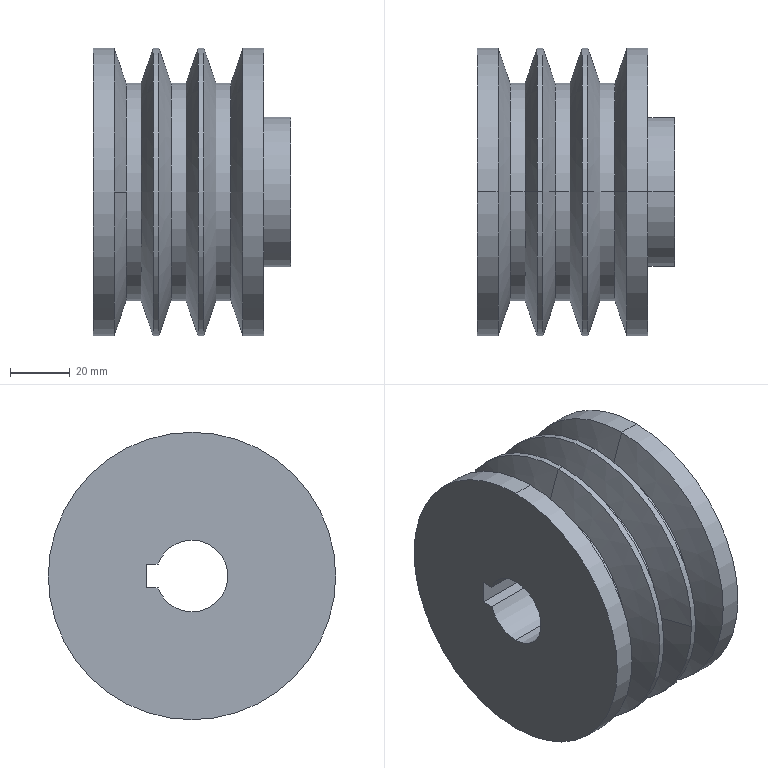Part | SolidWorks | features BaseBody 1 | 1 solid | 37 faces | box 66 x 96 x 96 mm | volume 312790 mm3 | cylinder 19 | cone 12 | plane 6 | commonest cylinder face diameters 96 x8 72.6 x6 24 x3 50 x2
STEP:
#1=CARTESIAN_POINT('',(-28.5,0.,48.));
#2=VERTEX_POINT('',#1);
#3=CARTESIAN_POINT('',(-28.5,0.,-48.));
#4=VERTEX_POINT('',#3);
#5=CARTESIAN_POINT('',(-28.5,0.,0.));
#6=DIRECTION('',(-1.,0.,0.));
#7=DIRECTION('',(0.,0.,-1.));
#8=AXIS2_PLACEMENT_3D('',#5,#6,#7);
#9=CIRCLE('',#8,48.);
#10=EDGE_CURVE('',#2,#4,#9,.T.);
#11=ORIENTED_EDGE('',*,*,#10,.F.);
#12=CARTESIAN_POINT('',(-21.533,0.,48.));
#13=VERTEX_POINT('',#12);
#14=CARTESIAN_POINT('',(0.,0.,48.));
#15=DIRECTION('',(1.,0.,0.));
#16=VECTOR('',#15,1000.);
#17=LINE('',#14,#16);
#18=EDGE_CURVE('',#2,#13,#17,.T.);
#19=ORIENTED_EDGE('',*,*,#18,.T.);
#20=CARTESIAN_POINT('',(-21.533,48.,0.));
#21=VERTEX_POINT('',#20);
#22=CARTESIAN_POINT('',(-21.533,0.,0.));
#23=DIRECTION('',(-1.,0.,0.));
#24=DIRECTION('',(0.,0.,-1.));
#25=AXIS2_PLACEMENT_3D('',#22,#23,#24);
#26=CIRCLE('',#25,48.);
#27=EDGE_CURVE('',#13,#21,#26,.T.);
#28=ORIENTED_EDGE('',*,*,#27,.T.);
#29=CARTESIAN_POINT('',(-21.533,0.,-48.));
#30=VERTEX_POINT('',#29);
#31=CARTESIAN_POINT('',(-21.533,0.,0.));
#32=DIRECTION('',(-1.,0.,0.));
#33=DIRECTION('',(0.,0.,-1.));
#34=AXIS2_PLACEMENT_3D('',#31,#32,#33);
#35=CIRCLE('',#34,48.);
#36=EDGE_CURVE('',#21,#30,#35,.T.);
#37=ORIENTED_EDGE('',*,*,#36,.T.);
#38=CARTESIAN_POINT('',(0.,0.,-48.));
#39=DIRECTION('',(1.,0.,0.));
#40=VECTOR('',#39,1000.);
#41=LINE('',#38,#40);
#42=EDGE_CURVE('',#4,#30,#41,.T.);
#43=ORIENTED_EDGE('',*,*,#42,.F.);
#44=EDGE_LOOP('',(#11,#19,#28,#37,#43));
#45=FACE_OUTER_BOUND('',#44,.T.);
#46=CARTESIAN_POINT('',(0.,0.,0.));
#47=DIRECTION('',(1.,0.,0.));
#48=DIRECTION('',(0.,0.,-1.));
#49=AXIS2_PLACEMENT_3D('',#46,#47,#48);
#50=CYLINDRICAL_SURFACE('',#49,48.);
#51=ADVANCED_FACE('',(#45),#50,.T.);
#52=CARTESIAN_POINT('',(-28.5,0.,12.));
#53=VERTEX_POINT('',#52);
#54=CARTESIAN_POINT('',(-28.5,0.,-12.));
#55=VERTEX_POINT('',#54);
#56=CARTESIAN_POINT('',(-28.5,0.,0.));
#57=DIRECTION('',(1.,0.,0.));
#58=DIRECTION('',(0.,0.,-1.));
#59=AXIS2_PLACEMENT_3D('',#56,#57,#58);
#60=CIRCLE('',#59,12.);
#61=EDGE_CURVE('',#53,#55,#60,.T.);
#62=ORIENTED_EDGE('',*,*,#61,.F.);
#63=CARTESIAN_POINT('',(37.5,0.,12.));
#64=VERTEX_POINT('',#63);
#65=CARTESIAN_POINT('',(0.,0.,12.));
#66=DIRECTION('',(1.,0.,0.));
#67=VECTOR('',#66,1000.);
#68=LINE('',#65,#67);
#69=EDGE_CURVE('',#53,#64,#68,.T.);
#70=ORIENTED_EDGE('',*,*,#69,.T.);
#71=CARTESIAN_POINT('',(37.5,0.,-12.));
#72=VERTEX_POINT('',#71);
#73=CARTESIAN_POINT('',(37.5,0.,0.));
#74=DIRECTION('',(-1.,0.,0.));
#75=DIRECTION('',(0.,0.,-1.));
#76=AXIS2_PLACEMENT_3D('',#73,#74,#75);
#77=CIRCLE('',#76,12.);
#78=EDGE_CURVE('',#72,#64,#77,.T.);
#79=ORIENTED_EDGE('',*,*,#78,.F.);
#80=CARTESIAN_POINT('',(0.,0.,-12.));
#81=DIRECTION('',(1.,0.,0.));
#82=VECTOR('',#81,1000.);
#83=LINE('',#80,#82);
#84=EDGE_CURVE('',#55,#72,#83,.T.);
#85=ORIENTED_EDGE('',*,*,#84,.F.);
#86=EDGE_LOOP('',(#62,#70,#79,#85));
#87=FACE_OUTER_BOUND('',#86,.T.);
#88=CARTESIAN_POINT('',(0.,0.,0.));
#89=DIRECTION('',(1.,0.,0.));
#90=DIRECTION('',(0.,0.,-1.));
#91=AXIS2_PLACEMENT_3D('',#88,#89,#90);
#92=CYLINDRICAL_SURFACE('',#91,12.);
#93=ADVANCED_FACE('',(#87),#92,.F.);
#94=CARTESIAN_POINT('',(-28.5,11.314,-4.));
#95=VERTEX_POINT('',#94);
#96=CARTESIAN_POINT('',(-28.5,0.,0.));
#97=DIRECTION('',(1.,0.,0.));
#98=DIRECTION('',(0.,0.,-1.));
#99=AXIS2_PLACEMENT_3D('',#96,#97,#98);
#100=CIRCLE('',#99,12.);
#101=EDGE_CURVE('',#55,#95,#100,.T.);
#102=ORIENTED_EDGE('',*,*,#101,.F.);
#103=ORIENTED_EDGE('',*,*,#84,.T.);
#104=CARTESIAN_POINT('',(37.5,11.314,-4.));
#105=VERTEX_POINT('',#104);
#106=CARTESIAN_POINT('',(37.5,0.,0.));
#107=DIRECTION('',(-1.,0.,0.));
#108=DIRECTION('',(0.,0.,-1.));
#109=AXIS2_PLACEMENT_3D('',#106,#107,#108);
#110=CIRCLE('',#109,12.);
#111=EDGE_CURVE('',#105,#72,#110,.T.);
#112=ORIENTED_EDGE('',*,*,#111,.F.);
#113=CARTESIAN_POINT('',(0.,11.314,-4.));
#114=DIRECTION('',(1.,0.,0.));
#115=VECTOR('',#114,1000.);
#116=LINE('',#113,#115);
#117=EDGE_CURVE('',#95,#105,#116,.T.);
#118=ORIENTED_EDGE('',*,*,#117,.F.);
#119=EDGE_LOOP('',(#102,#103,#112,#118));
#120=FACE_OUTER_BOUND('',#119,.T.);
#121=CARTESIAN_POINT('',(0.,0.,0.));
#122=DIRECTION('',(1.,0.,0.));
#123=DIRECTION('',(0.,0.,-1.));
#124=AXIS2_PLACEMENT_3D('',#121,#122,#123);
#125=CYLINDRICAL_SURFACE('',#124,12.);
#126=ADVANCED_FACE('',(#120),#125,.F.);
#127=CARTESIAN_POINT('',(-17.504,0.,36.3));
#128=VERTEX_POINT('',#127);
#129=CARTESIAN_POINT('',(-17.504,36.3,0.));
#130=VERTEX_POINT('',#129);
#131=CARTESIAN_POINT('',(-17.504,0.,0.));
#132=DIRECTION('',(-1.,0.,0.));
#133=DIRECTION('',(0.,0.,1.));
#134=AXIS2_PLACEMENT_3D('',#131,#132,#133);
#135=CIRCLE('',#134,36.3);
#136=EDGE_CURVE('',#128,#130,#135,.T.);
#137=ORIENTED_EDGE('',*,*,#136,.T.);
#138=CARTESIAN_POINT('',(-21.533,48.,0.));
#139=DIRECTION('',(-0.3256,0.9455,0.));
#140=VECTOR('',#139,1000.);
#141=LINE('',#138,#140);
#142=EDGE_CURVE('',#130,#21,#141,.T.);
#143=ORIENTED_EDGE('',*,*,#142,.T.);
#144=ORIENTED_EDGE('',*,*,#27,.F.);
#145=CARTESIAN_POINT('',(-21.533,-48.,0.));
#146=VERTEX_POINT('',#145);
#147=CARTESIAN_POINT('',(-21.533,0.,0.));
#148=DIRECTION('',(-1.,0.,0.));
#149=DIRECTION('',(0.,0.,-1.));
#150=AXIS2_PLACEMENT_3D('',#147,#148,#149);
#151=CIRCLE('',#150,48.);
#152=EDGE_CURVE('',#146,#13,#151,.T.);
#153=ORIENTED_EDGE('',*,*,#152,.F.);
#154=CARTESIAN_POINT('',(-17.504,-36.3,0.));
#155=VERTEX_POINT('',#154);
#156=CARTESIAN_POINT('',(-21.533,-48.,0.));
#157=DIRECTION('',(-0.3256,-0.9455,0.));
#158=VECTOR('',#157,1000.);
#159=LINE('',#156,#158);
#160=EDGE_CURVE('',#155,#146,#159,.T.);
#161=ORIENTED_EDGE('',*,*,#160,.F.);
#162=CARTESIAN_POINT('',(-17.504,0.,0.));
#163=DIRECTION('',(-1.,0.,0.));
#164=DIRECTION('',(0.,0.,1.));
#165=AXIS2_PLACEMENT_3D('',#162,#163,#164);
#166=CIRCLE('',#165,36.3);
#167=EDGE_CURVE('',#155,#128,#166,.T.);
#168=ORIENTED_EDGE('',*,*,#167,.T.);
#169=EDGE_LOOP('',(#137,#143,#144,#153,#161,#168));
#170=FACE_OUTER_BOUND('',#169,.T.);
#171=CARTESIAN_POINT('',(-21.533,0.,0.));
#172=DIRECTION('',(-1.,0.,0.));
#173=DIRECTION('',(0.,-1.,0.));
#174=AXIS2_PLACEMENT_3D('',#171,#172,#173);
#175=CONICAL_SURFACE('',#174,48.,1.239);
#176=ADVANCED_FACE('',(#170),#175,.T.);
#177=CARTESIAN_POINT('',(-12.496,0.,36.3));
#178=VERTEX_POINT('',#177);
#179=CARTESIAN_POINT('',(-12.496,0.,-36.3));
#180=VERTEX_POINT('',#179);
#181=CARTESIAN_POINT('',(-12.496,0.,0.));
#182=DIRECTION('',(-1.,0.,0.));
#183=DIRECTION('',(0.,0.,1.));
#184=AXIS2_PLACEMENT_3D('',#181,#182,#183);
#185=CIRCLE('',#184,36.3);
#186=EDGE_CURVE('',#178,#180,#185,.T.);
#187=ORIENTED_EDGE('',*,*,#186,.T.);
#188=CARTESIAN_POINT('',(-17.504,0.,-36.3));
#189=VERTEX_POINT('',#188);
#190=CARTESIAN_POINT('',(-15.,0.,-36.3));
#191=DIRECTION('',(-1.,0.,0.));
#192=VECTOR('',#191,1000.);
#193=LINE('',#190,#192);
#194=EDGE_CURVE('',#180,#189,#193,.T.);
#195=ORIENTED_EDGE('',*,*,#194,.T.);
#196=CARTESIAN_POINT('',(-17.504,0.,0.));
#197=DIRECTION('',(-1.,0.,0.));
#198=DIRECTION('',(0.,0.,1.));
#199=AXIS2_PLACEMENT_3D('',#196,#197,#198);
#200=CIRCLE('',#199,36.3);
#201=EDGE_CURVE('',#130,#189,#200,.T.);
#202=ORIENTED_EDGE('',*,*,#201,.F.);
#203=ORIENTED_EDGE('',*,*,#136,.F.);
#204=CARTESIAN_POINT('',(-15.,0.,36.3));
#205=DIRECTION('',(-1.,0.,0.));
#206=VECTOR('',#205,1000.);
#207=LINE('',#204,#206);
#208=EDGE_CURVE('',#178,#128,#207,.T.);
#209=ORIENTED_EDGE('',*,*,#208,.F.);
#210=EDGE_LOOP('',(#187,#195,#202,#203,#209));
#211=FACE_OUTER_BOUND('',#210,.T.);
#212=CARTESIAN_POINT('',(-15.,0.,0.));
#213=DIRECTION('',(-1.,0.,0.));
#214=DIRECTION('',(0.,0.,1.));
#215=AXIS2_PLACEMENT_3D('',#212,#213,#214);
#216=CYLINDRICAL_SURFACE('',#215,36.3);
#217=ADVANCED_FACE('',(#211),#216,.T.);
#218=CARTESIAN_POINT('',(28.5,0.,-25.));
#219=VERTEX_POINT('',#218);
#220=CARTESIAN_POINT('',(28.5,0.,25.));
#221=VERTEX_POINT('',#220);
#222=CARTESIAN_POINT('',(28.5,0.,0.));
#223=DIRECTION('',(1.,0.,0.));
#224=DIRECTION('',(0.,0.,-1.));
#225=AXIS2_PLACEMENT_3D('',#222,#223,#224);
#226=CIRCLE('',#225,25.);
#227=EDGE_CURVE('',#219,#221,#226,.T.);
#228=ORIENTED_EDGE('',*,*,#227,.T.);
#229=CARTESIAN_POINT('',(37.5,0.,25.));
#230=VERTEX_POINT('',#229);
#231=CARTESIAN_POINT('',(0.,0.,25.));
#232=DIRECTION('',(1.,0.,0.));
#233=VECTOR('',#232,1000.);
#234=LINE('',#231,#233);
#235=EDGE_CURVE('',#221,#230,#234,.T.);
#236=ORIENTED_EDGE('',*,*,#235,.T.);
#237=CARTESIAN_POINT('',(37.5,0.,-25.));
#238=VERTEX_POINT('',#237);
#239=CARTESIAN_POINT('',(37.5,0.,0.));
#240=DIRECTION('',(1.,0.,0.));
#241=DIRECTION('',(0.,0.,-1.));
#242=AXIS2_PLACEMENT_3D('',#239,#240,#241);
#243=CIRCLE('',#242,25.);
#244=EDGE_CURVE('',#238,#230,#243,.T.);
#245=ORIENTED_EDGE('',*,*,#244,.F.);
#246=CARTESIAN_POINT('',(0.,0.,-25.));
#247=DIRECTION('',(1.,0.,0.));
#248=VECTOR('',#247,1000.);
#249=LINE('',#246,#248);
#250=EDGE_CURVE('',#219,#238,#249,.T.);
#251=ORIENTED_EDGE('',*,*,#250,.F.);
#252=EDGE_LOOP('',(#228,#236,#245,#251));
#253=FACE_OUTER_BOUND('',#252,.T.);
#254=CARTESIAN_POINT('',(0.,0.,0.));
#255=DIRECTION('',(1.,0.,0.));
#256=DIRECTION('',(0.,0.,-1.));
#257=AXIS2_PLACEMENT_3D('',#254,#255,#256);
#258=CYLINDRICAL_SURFACE('',#257,25.);
#259=ADVANCED_FACE('',(#253),#258,.T.);
#260=ORIENTED_EDGE('',*,*,#186,.F.);
#261=CARTESIAN_POINT('',(-8.467,0.,48.));
#262=VERTEX_POINT('',#261);
#263=CARTESIAN_POINT('',(-8.467,0.,48.));
#264=DIRECTION('',(0.3256,0.,0.9455));
#265=VECTOR('',#264,1000.);
#266=LINE('',#263,#265);
#267=EDGE_CURVE('',#178,#262,#266,.T.);
#268=ORIENTED_EDGE('',*,*,#267,.T.);
#269=CARTESIAN_POINT('',(-8.467,0.,-48.));
#270=VERTEX_POINT('',#269);
#271=CARTESIAN_POINT('',(-8.467,0.,0.));
#272=DIRECTION('',(-1.,0.,0.));
#273=DIRECTION('',(0.,0.,-1.));
#274=AXIS2_PLACEMENT_3D('',#271,#272,#273);
#275=CIRCLE('',#274,48.);
#276=EDGE_CURVE('',#262,#270,#275,.T.);
#277=ORIENTED_EDGE('',*,*,#276,.T.);
#278=CARTESIAN_POINT('',(-8.467,0.,-48.));
#279=DIRECTION('',(0.3256,0.,-0.9455));
#280=VECTOR('',#279,1000.);
#281=LINE('',#278,#280);
#282=EDGE_CURVE('',#180,#270,#281,.T.);
#283=ORIENTED_EDGE('',*,*,#282,.F.);
#284=EDGE_LOOP('',(#260,#268,#277,#283));
#285=FACE_OUTER_BOUND('',#284,.T.);
#286=CARTESIAN_POINT('',(-8.467,0.,0.));
#287=DIRECTION('',(1.,0.,0.));
#288=DIRECTION('',(0.,0.,-1.));
#289=AXIS2_PLACEMENT_3D('',#286,#287,#288);
#290=CONICAL_SURFACE('',#289,48.,1.239);
#291=ADVANCED_FACE('',(#285),#290,.T.);
#292=ORIENTED_EDGE('',*,*,#276,.F.);
#293=CARTESIAN_POINT('',(-6.533,0.,48.));
#294=VERTEX_POINT('',#293);
#295=CARTESIAN_POINT('',(0.,0.,48.));
#296=DIRECTION('',(1.,0.,0.));
#297=VECTOR('',#296,1000.);
#298=LINE('',#295,#297);
#299=EDGE_CURVE('',#262,#294,#298,.T.);
#300=ORIENTED_EDGE('',*,*,#299,.T.);
#301=CARTESIAN_POINT('',(-6.533,0.,-48.));
#302=VERTEX_POINT('',#301);
#303=CARTESIAN_POINT('',(-6.533,0.,0.));
#304=DIRECTION('',(-1.,0.,0.));
#305=DIRECTION('',(0.,0.,-1.));
#306=AXIS2_PLACEMENT_3D('',#303,#304,#305);
#307=CIRCLE('',#306,48.);
#308=EDGE_CURVE('',#294,#302,#307,.T.);
#309=ORIENTED_EDGE('',*,*,#308,.T.);
#310=CARTESIAN_POINT('',(0.,0.,-48.));
#311=DIRECTION('',(1.,0.,0.));
#312=VECTOR('',#311,1000.);
#313=LINE('',#310,#312);
#314=EDGE_CURVE('',#270,#302,#313,.T.);
#315=ORIENTED_EDGE('',*,*,#314,.F.);
#316=EDGE_LOOP('',(#292,#300,#309,#315));
#317=FACE_OUTER_BOUND('',#316,.T.);
#318=CARTESIAN_POINT('',(0.,0.,0.));
#319=DIRECTION('',(1.,0.,0.));
#320=DIRECTION('',(0.,0.,-1.));
#321=AXIS2_PLACEMENT_3D('',#318,#319,#320);
#322=CYLINDRICAL_SURFACE('',#321,48.);
#323=ADVANCED_FACE('',(#317),#322,.T.);
#324=CARTESIAN_POINT('',(21.533,0.,-48.));
#325=VERTEX_POINT('',#324);
#326=CARTESIAN_POINT('',(21.533,0.,48.));
#327=VERTEX_POINT('',#326);
#328=CARTESIAN_POINT('',(21.533,0.,0.));
#329=DIRECTION('',(1.,0.,0.));
#330=DIRECTION('',(0.,0.,-1.));
#331=AXIS2_PLACEMENT_3D('',#328,#329,#330);
#332=CIRCLE('',#331,48.);
#333=EDGE_CURVE('',#325,#327,#332,.T.);
#334=ORIENTED_EDGE('',*,*,#333,.T.);
#335=CARTESIAN_POINT('',(28.5,0.,48.));
#336=VERTEX_POINT('',#335);
#337=CARTESIAN_POINT('',(0.,0.,48.));
#338=DIRECTION('',(1.,0.,0.));
#339=VECTOR('',#338,1000.);
#340=LINE('',#337,#339);
#341=EDGE_CURVE('',#327,#336,#340,.T.);
#342=ORIENTED_EDGE('',*,*,#341,.T.);
#343=CARTESIAN_POINT('',(28.5,0.,-48.));
#344=VERTEX_POINT('',#343);
#345=CARTESIAN_POINT('',(28.5,0.,0.));
#346=DIRECTION('',(1.,0.,0.));
#347=DIRECTION('',(0.,0.,-1.));
#348=AXIS2_PLACEMENT_3D('',#345,#346,#347);
#349=CIRCLE('',#348,48.);
#350=EDGE_CURVE('',#344,#336,#349,.T.);
#351=ORIENTED_EDGE('',*,*,#350,.F.);
#352=CARTESIAN_POINT('',(0.,0.,-48.));
#353=DIRECTION('',(1.,0.,0.));
#354=VECTOR('',#353,1000.);
#355=LINE('',#352,#354);
#356=EDGE_CURVE('',#325,#344,#355,.T.);
#357=ORIENTED_EDGE('',*,*,#356,.F.);
#358=EDGE_LOOP('',(#334,#342,#351,#357));
#359=FACE_OUTER_BOUND('',#358,.T.);
#360=CARTESIAN_POINT('',(0.,0.,0.));
#361=DIRECTION('',(1.,0.,0.));
#362=DIRECTION('',(0.,0.,-1.));
#363=AXIS2_PLACEMENT_3D('',#360,#361,#362);
#364=CYLINDRICAL_SURFACE('',#363,48.);
#365=ADVANCED_FACE('',(#359),#364,.T.);
#366=CARTESIAN_POINT('',(-2.504,0.,36.3));
#367=VERTEX_POINT('',#366);
#368=CARTESIAN_POINT('',(-2.504,0.,-36.3));
#369=VERTEX_POINT('',#368);
#370=CARTESIAN_POINT('',(-2.504,0.,0.));
#371=DIRECTION('',(-1.,0.,0.));
#372=DIRECTION('',(0.,0.,1.));
#373=AXIS2_PLACEMENT_3D('',#370,#371,#372);
#374=CIRCLE('',#373,36.3);
#375=EDGE_CURVE('',#367,#369,#374,.T.);
#376=ORIENTED_EDGE('',*,*,#375,.T.);
#377=CARTESIAN_POINT('',(-6.533,0.,-48.));
#378=DIRECTION('',(-0.3256,0.,-0.9455));
#379=VECTOR('',#378,1000.);
#380=LINE('',#377,#379);
#381=EDGE_CURVE('',#369,#302,#380,.T.);
#382=ORIENTED_EDGE('',*,*,#381,.T.);
#383=ORIENTED_EDGE('',*,*,#308,.F.);
#384=CARTESIAN_POINT('',(-6.533,0.,48.));
#385=DIRECTION('',(-0.3256,0.,0.9455));
#386=VECTOR('',#385,1000.);
#387=LINE('',#384,#386);
#388=EDGE_CURVE('',#367,#294,#387,.T.);
#389=ORIENTED_EDGE('',*,*,#388,.F.);
#390=EDGE_LOOP('',(#376,#382,#383,#389));
#391=FACE_OUTER_BOUND('',#390,.T.);
#392=CARTESIAN_POINT('',(-6.533,0.,0.));
#393=DIRECTION('',(-1.,0.,0.));
#394=DIRECTION('',(0.,0.,1.));
#395=AXIS2_PLACEMENT_3D('',#392,#393,#394);
#396=CONICAL_SURFACE('',#395,48.,1.239);
#397=ADVANCED_FACE('',(#391),#396,.T.);
#398=CARTESIAN_POINT('',(17.504,0.,-36.3));
#399=VERTEX_POINT('',#398);
#400=CARTESIAN_POINT('',(17.504,0.,36.3));
#401=VERTEX_POINT('',#400);
#402=CARTESIAN_POINT('',(17.504,0.,0.));
#403=DIRECTION('',(1.,0.,0.));
#404=DIRECTION('',(0.,0.,-1.));
#405=AXIS2_PLACEMENT_3D('',#402,#403,#404);
#406=CIRCLE('',#405,36.3);
#407=EDGE_CURVE('',#399,#401,#406,.T.);
#408=ORIENTED_EDGE('',*,*,#407,.T.);
#409=CARTESIAN_POINT('',(21.533,0.,48.));
#410=DIRECTION('',(0.3256,0.,0.9455));
#411=VECTOR('',#410,1000.);
#412=LINE('',#409,#411);
#413=EDGE_CURVE('',#401,#327,#412,.T.);
#414=ORIENTED_EDGE('',*,*,#413,.T.);
#415=ORIENTED_EDGE('',*,*,#333,.F.);
#416=CARTESIAN_POINT('',(21.533,0.,-48.));
#417=DIRECTION('',(0.3256,0.,-0.9455));
#418=VECTOR('',#417,1000.);
#419=LINE('',#416,#418);
#420=EDGE_CURVE('',#399,#325,#419,.T.);
#421=ORIENTED_EDGE('',*,*,#420,.F.);
#422=EDGE_LOOP('',(#408,#414,#415,#421));
#423=FACE_OUTER_BOUND('',#422,.T.);
#424=CARTESIAN_POINT('',(21.533,0.,0.));
#425=DIRECTION('',(1.,0.,0.));
#426=DIRECTION('',(0.,0.,-1.));
#427=AXIS2_PLACEMENT_3D('',#424,#425,#426);
#428=CONICAL_SURFACE('',#427,48.,1.239);
#429=ADVANCED_FACE('',(#423),#428,.T.);
#430=CARTESIAN_POINT('',(2.504,36.3,0.));
#431=VERTEX_POINT('',#430);
#432=CARTESIAN_POINT('',(2.504,0.,-36.3));
#433=VERTEX_POINT('',#432);
#434=CARTESIAN_POINT('',(2.504,0.,0.));
#435=DIRECTION('',(-1.,0.,0.));
#436=DIRECTION('',(0.,0.,1.));
#437=AXIS2_PLACEMENT_3D('',#434,#435,#436);
#438=CIRCLE('',#437,36.3);
#439=EDGE_CURVE('',#431,#433,#438,.T.);
#440=ORIENTED_EDGE('',*,*,#439,.T.);
#441=CARTESIAN_POINT('',(0.,0.,-36.3));
#442=DIRECTION('',(-1.,0.,0.));
#443=VECTOR('',#442,1000.);
#444=LINE('',#441,#443);
#445=EDGE_CURVE('',#433,#369,#444,.T.);
#446=ORIENTED_EDGE('',*,*,#445,.T.);
#447=ORIENTED_EDGE('',*,*,#375,.F.);
#448=CARTESIAN_POINT('',(2.504,0.,36.3));
#449=VERTEX_POINT('',#448);
#450=CARTESIAN_POINT('',(0.,0.,36.3));
#451=DIRECTION('',(-1.,0.,0.));
#452=VECTOR('',#451,1000.);
#453=LINE('',#450,#452);
#454=EDGE_CURVE('',#449,#367,#453,.T.);
#455=ORIENTED_EDGE('',*,*,#454,.F.);
#456=CARTESIAN_POINT('',(2.504,0.,0.));
#457=DIRECTION('',(-1.,0.,0.));
#458=DIRECTION('',(0.,0.,1.));
#459=AXIS2_PLACEMENT_3D('',#456,#457,#458);
#460=CIRCLE('',#459,36.3);
#461=EDGE_CURVE('',#449,#431,#460,.T.);
#462=ORIENTED_EDGE('',*,*,#461,.T.);
#463=EDGE_LOOP('',(#440,#446,#447,#455,#462));
#464=FACE_OUTER_BOUND('',#463,.T.);
#465=CARTESIAN_POINT('',(0.,0.,0.));
#466=DIRECTION('',(-1.,0.,0.));
#467=DIRECTION('',(0.,0.,1.));
#468=AXIS2_PLACEMENT_3D('',#465,#466,#467);
#469=CYLINDRICAL_SURFACE('',#468,36.3);
#470=ADVANCED_FACE('',(#464),#469,.T.);
#471=ORIENTED_EDGE('',*,*,#407,.F.);
#472=CARTESIAN_POINT('',(12.496,0.,-36.3));
#473=VERTEX_POINT('',#472);
#474=CARTESIAN_POINT('',(15.,0.,-36.3));
#475=DIRECTION('',(-1.,0.,0.));
#476=VECTOR('',#475,1000.);
#477=LINE('',#474,#476);
#478=EDGE_CURVE('',#399,#473,#477,.T.);
#479=ORIENTED_EDGE('',*,*,#478,.T.);
#480=CARTESIAN_POINT('',(12.496,0.,36.3));
#481=VERTEX_POINT('',#480);
#482=CARTESIAN_POINT('',(12.496,0.,0.));
#483=DIRECTION('',(1.,0.,0.));
#484=DIRECTION('',(0.,0.,1.));
#485=AXIS2_PLACEMENT_3D('',#482,#483,#484);
#486=CIRCLE('',#485,36.3);
#487=EDGE_CURVE('',#473,#481,#486,.T.);
#488=ORIENTED_EDGE('',*,*,#487,.T.);
#489=CARTESIAN_POINT('',(15.,0.,36.3));
#490=DIRECTION('',(-1.,0.,0.));
#491=VECTOR('',#490,1000.);
#492=LINE('',#489,#491);
#493=EDGE_CURVE('',#401,#481,#492,.T.);
#494=ORIENTED_EDGE('',*,*,#493,.F.);
#495=EDGE_LOOP('',(#471,#479,#488,#494));
#496=FACE_OUTER_BOUND('',#495,.T.);
#497=CARTESIAN_POINT('',(15.,0.,0.));
#498=DIRECTION('',(-1.,0.,0.));
#499=DIRECTION('',(0.,0.,1.));
#500=AXIS2_PLACEMENT_3D('',#497,#498,#499);
#501=CYLINDRICAL_SURFACE('',#500,36.3);
#502=ADVANCED_FACE('',(#496),#501,.T.);
#503=CARTESIAN_POINT('',(2.504,-36.3,0.));
#504=VERTEX_POINT('',#503);
#505=CARTESIAN_POINT('',(2.504,0.,0.));
#506=DIRECTION('',(-1.,0.,0.));
#507=DIRECTION('',(0.,0.,1.));
#508=AXIS2_PLACEMENT_3D('',#505,#506,#507);
#509=CIRCLE('',#508,36.3);
#510=EDGE_CURVE('',#504,#449,#509,.T.);
#511=ORIENTED_EDGE('',*,*,#510,.F.);
#512=CARTESIAN_POINT('',(6.533,-48.,0.));
#513=VERTEX_POINT('',#512);
#514=CARTESIAN_POINT('',(6.533,-48.,0.));
#515=DIRECTION('',(0.3256,-0.9455,0.));
#516=VECTOR('',#515,1000.);
#517=LINE('',#514,#516);
#518=EDGE_CURVE('',#504,#513,#517,.T.);
#519=ORIENTED_EDGE('',*,*,#518,.T.);
#520=CARTESIAN_POINT('',(6.533,0.,48.));
#521=VERTEX_POINT('',#520);
#522=CARTESIAN_POINT('',(6.533,0.,0.));
#523=DIRECTION('',(-1.,0.,0.));
#524=DIRECTION('',(0.,0.,-1.));
#525=AXIS2_PLACEMENT_3D('',#522,#523,#524);
#526=CIRCLE('',#525,48.);
#527=EDGE_CURVE('',#513,#521,#526,.T.);
#528=ORIENTED_EDGE('',*,*,#527,.T.);
#529=CARTESIAN_POINT('',(6.533,48.,0.));
#530=VERTEX_POINT('',#529);
#531=CARTESIAN_POINT('',(6.533,0.,0.));
#532=DIRECTION('',(-1.,0.,0.));
#533=DIRECTION('',(0.,0.,-1.));
#534=AXIS2_PLACEMENT_3D('',#531,#532,#533);
#535=CIRCLE('',#534,48.);
#536=EDGE_CURVE('',#521,#530,#535,.T.);
#537=ORIENTED_EDGE('',*,*,#536,.T.);
#538=CARTESIAN_POINT('',(6.533,48.,0.));
#539=DIRECTION('',(0.3256,0.9455,0.));
#540=VECTOR('',#539,1000.);
#541=LINE('',#538,#540);
#542=EDGE_CURVE('',#431,#530,#541,.T.);
#543=ORIENTED_EDGE('',*,*,#542,.F.);
#544=ORIENTED_EDGE('',*,*,#461,.F.);
#545=EDGE_LOOP('',(#511,#519,#528,#537,#543,#544));
#546=FACE_OUTER_BOUND('',#545,.T.);
#547=CARTESIAN_POINT('',(6.533,0.,0.));
#548=DIRECTION('',(1.,0.,0.));
#549=DIRECTION('',(0.,1.,0.));
#550=AXIS2_PLACEMENT_3D('',#547,#548,#549);
#551=CONICAL_SURFACE('',#550,48.,1.239);
#552=ADVANCED_FACE('',(#546),#551,.T.);
#553=ORIENTED_EDGE('',*,*,#487,.F.);
#554=CARTESIAN_POINT('',(8.467,0.,-48.));
#555=VERTEX_POINT('',#554);
#556=CARTESIAN_POINT('',(8.467,0.,-48.));
#557=DIRECTION('',(-0.3256,0.,-0.9455));
#558=VECTOR('',#557,1000.);
#559=LINE('',#556,#558);
#560=EDGE_CURVE('',#473,#555,#559,.T.);
#561=ORIENTED_EDGE('',*,*,#560,.T.);
#562=CARTESIAN_POINT('',(8.467,0.,48.));
#563=VERTEX_POINT('',#562);
#564=CARTESIAN_POINT('',(8.467,0.,0.));
#565=DIRECTION('',(1.,0.,0.));
#566=DIRECTION('',(0.,0.,1.));
#567=AXIS2_PLACEMENT_3D('',#564,#565,#566);
#568=CIRCLE('',#567,48.);
#569=EDGE_CURVE('',#555,#563,#568,.T.);
#570=ORIENTED_EDGE('',*,*,#569,.T.);
#571=CARTESIAN_POINT('',(8.467,0.,48.));
#572=DIRECTION('',(-0.3256,0.,0.9455));
#573=VECTOR('',#572,1000.);
#574=LINE('',#571,#573);
#575=EDGE_CURVE('',#481,#563,#574,.T.);
#576=ORIENTED_EDGE('',*,*,#575,.F.);
#577=EDGE_LOOP('',(#553,#561,#570,#576));
#578=FACE_OUTER_BOUND('',#577,.T.);
#579=CARTESIAN_POINT('',(8.467,0.,0.));
#580=DIRECTION('',(-1.,0.,0.));
#581=DIRECTION('',(0.,0.,1.));
#582=AXIS2_PLACEMENT_3D('',#579,#580,#581);
#583=CONICAL_SURFACE('',#582,48.,1.239);
#584=ADVANCED_FACE('',(#578),#583,.T.);
#585=ORIENTED_EDGE('',*,*,#536,.F.);
#586=CARTESIAN_POINT('',(0.,0.,48.));
#587=DIRECTION('',(1.,0.,0.));
#588=VECTOR('',#587,1000.);
#589=LINE('',#586,#588);
#590=EDGE_CURVE('',#521,#563,#589,.T.);
#591=ORIENTED_EDGE('',*,*,#590,.T.);
#592=ORIENTED_EDGE('',*,*,#569,.F.);
#593=CARTESIAN_POINT('',(6.533,0.,-48.));
#594=VERTEX_POINT('',#593);
#595=CARTESIAN_POINT('',(0.,0.,-48.));
#596=DIRECTION('',(1.,0.,0.));
#597=VECTOR('',#596,1000.);
#598=LINE('',#595,#597);
#599=EDGE_CURVE('',#594,#555,#598,.T.);
#600=ORIENTED_EDGE('',*,*,#599,.F.);
#601=CARTESIAN_POINT('',(6.533,0.,0.));
#602=DIRECTION('',(-1.,0.,0.));
#603=DIRECTION('',(0.,0.,-1.));
#604=AXIS2_PLACEMENT_3D('',#601,#602,#603);
#605=CIRCLE('',#604,48.);
#606=EDGE_CURVE('',#530,#594,#605,.T.);
#607=ORIENTED_EDGE('',*,*,#606,.F.);
#608=EDGE_LOOP('',(#585,#591,#592,#600,#607));
#609=FACE_OUTER_BOUND('',#608,.T.);
#610=CARTESIAN_POINT('',(0.,0.,0.));
#611=DIRECTION('',(1.,0.,0.));
#612=DIRECTION('',(0.,0.,-1.));
#613=AXIS2_PLACEMENT_3D('',#610,#611,#612);
#614=CYLINDRICAL_SURFACE('',#613,48.);
#615=ADVANCED_FACE('',(#609),#614,.T.);
#616=CARTESIAN_POINT('',(-28.5,0.,0.));
#617=DIRECTION('',(-1.,0.,0.));
#618=DIRECTION('',(0.,0.,-1.));
#619=AXIS2_PLACEMENT_3D('',#616,#617,#618);
#620=CIRCLE('',#619,48.);
#621=EDGE_CURVE('',#4,#2,#620,.T.);
#622=ORIENTED_EDGE('',*,*,#621,.T.);
#623=ORIENTED_EDGE('',*,*,#10,.T.);
#624=EDGE_LOOP('',(#622,#623));
#625=FACE_OUTER_BOUND('',#624,.T.);
#626=CARTESIAN_POINT('',(-28.5,11.314,4.));
#627=VERTEX_POINT('',#626);
#628=CARTESIAN_POINT('',(-28.5,0.,0.));
#629=DIRECTION('',(1.,0.,0.));
#630=DIRECTION('',(0.,0.,-1.));
#631=AXIS2_PLACEMENT_3D('',#628,#629,#630);
#632=CIRCLE('',#631,12.);
#633=EDGE_CURVE('',#627,#53,#632,.T.);
#634=ORIENTED_EDGE('',*,*,#633,.T.);
#635=ORIENTED_EDGE('',*,*,#61,.T.);
#636=ORIENTED_EDGE('',*,*,#101,.T.);
#637=CARTESIAN_POINT('',(-28.5,15.3,-4.));
#638=VERTEX_POINT('',#637);
#639=CARTESIAN_POINT('',(-28.5,48.,-4.));
#640=DIRECTION('',(0.,1.,0.));
#641=VECTOR('',#640,1000.);
#642=LINE('',#639,#641);
#643=EDGE_CURVE('',#95,#638,#642,.T.);
#644=ORIENTED_EDGE('',*,*,#643,.T.);
#645=CARTESIAN_POINT('',(-28.5,15.3,4.));
#646=VERTEX_POINT('',#645);
#647=CARTESIAN_POINT('',(-28.5,15.3,0.));
#648=DIRECTION('',(0.,0.,1.));
#649=VECTOR('',#648,1000.);
#650=LINE('',#647,#649);
#651=EDGE_CURVE('',#638,#646,#650,.T.);
#652=ORIENTED_EDGE('',*,*,#651,.T.);
#653=CARTESIAN_POINT('',(-28.5,48.,4.));
#654=DIRECTION('',(0.,-1.,0.));
#655=VECTOR('',#654,1000.);
#656=LINE('',#653,#655);
#657=EDGE_CURVE('',#646,#627,#656,.T.);
#658=ORIENTED_EDGE('',*,*,#657,.T.);
#659=EDGE_LOOP('',(#634,#635,#636,#644,#652,#658));
#660=FACE_BOUND('',#659,.T.);
#661=CARTESIAN_POINT('',(-28.5,48.,0.));
#662=DIRECTION('',(-1.,0.,0.));
#663=DIRECTION('',(0.,0.,1.));
#664=AXIS2_PLACEMENT_3D('',#661,#662,#663);
#665=PLANE('',#664);
#666=ADVANCED_FACE('',(#625,#660),#665,.T.);
#667=ORIENTED_EDGE('',*,*,#18,.F.);
#668=ORIENTED_EDGE('',*,*,#621,.F.);
#669=ORIENTED_EDGE('',*,*,#42,.T.);
#670=CARTESIAN_POINT('',(-21.533,0.,0.));
#671=DIRECTION('',(-1.,0.,0.));
#672=DIRECTION('',(0.,0.,-1.));
#673=AXIS2_PLACEMENT_3D('',#670,#671,#672);
#674=CIRCLE('',#673,48.);
#675=EDGE_CURVE('',#30,#146,#674,.T.);
#676=ORIENTED_EDGE('',*,*,#675,.T.);
#677=ORIENTED_EDGE('',*,*,#152,.T.);
#678=EDGE_LOOP('',(#667,#668,#669,#676,#677));
#679=FACE_OUTER_BOUND('',#678,.T.);
#680=CARTESIAN_POINT('',(0.,0.,0.));
#681=DIRECTION('',(1.,0.,0.));
#682=DIRECTION('',(0.,0.,-1.));
#683=AXIS2_PLACEMENT_3D('',#680,#681,#682);
#684=CYLINDRICAL_SURFACE('',#683,48.);
#685=ADVANCED_FACE('',(#679),#684,.T.);
#686=ORIENTED_EDGE('',*,*,#69,.F.);
#687=ORIENTED_EDGE('',*,*,#633,.F.);
#688=CARTESIAN_POINT('',(37.5,11.314,4.));
#689=VERTEX_POINT('',#688);
#690=CARTESIAN_POINT('',(0.,11.314,4.));
#691=DIRECTION('',(-1.,0.,0.));
#692=VECTOR('',#691,1000.);
#693=LINE('',#690,#692);
#694=EDGE_CURVE('',#689,#627,#693,.T.);
#695=ORIENTED_EDGE('',*,*,#694,.F.);
#696=CARTESIAN_POINT('',(37.5,0.,0.));
#697=DIRECTION('',(-1.,0.,0.));
#698=DIRECTION('',(0.,0.,-1.));
#699=AXIS2_PLACEMENT_3D('',#696,#697,#698);
#700=CIRCLE('',#699,12.);
#701=EDGE_CURVE('',#64,#689,#700,.T.);
#702=ORIENTED_EDGE('',*,*,#701,.F.);
#703=EDGE_LOOP('',(#686,#687,#695,#702));
#704=FACE_OUTER_BOUND('',#703,.T.);
#705=CARTESIAN_POINT('',(0.,0.,0.));
#706=DIRECTION('',(1.,0.,0.));
#707=DIRECTION('',(0.,0.,-1.));
#708=AXIS2_PLACEMENT_3D('',#705,#706,#707);
#709=CYLINDRICAL_SURFACE('',#708,12.);
#710=ADVANCED_FACE('',(#704),#709,.F.);
#711=ORIENTED_EDGE('',*,*,#657,.F.);
#712=CARTESIAN_POINT('',(37.5,15.3,4.));
#713=VERTEX_POINT('',#712);
#714=CARTESIAN_POINT('',(-28.5,15.3,4.));
#715=DIRECTION('',(-1.,0.,0.));
#716=VECTOR('',#715,1000.);
#717=LINE('',#714,#716);
#718=EDGE_CURVE('',#713,#646,#717,.T.);
#719=ORIENTED_EDGE('',*,*,#718,.F.);
#720=CARTESIAN_POINT('',(37.5,8.7,4.));
#721=DIRECTION('',(0.,1.,0.));
#722=VECTOR('',#721,1000.);
#723=LINE('',#720,#722);
#724=EDGE_CURVE('',#689,#713,#723,.T.);
#725=ORIENTED_EDGE('',*,*,#724,.F.);
#726=ORIENTED_EDGE('',*,*,#694,.T.);
#727=EDGE_LOOP('',(#711,#719,#725,#726));
#728=FACE_OUTER_BOUND('',#727,.T.);
#729=CARTESIAN_POINT('',(-28.5,8.7,4.));
#730=DIRECTION('',(0.,0.,1.));
#731=DIRECTION('',(1.,0.,0.));
#732=AXIS2_PLACEMENT_3D('',#729,#730,#731);
#733=PLANE('',#732);
#734=ADVANCED_FACE('',(#728),#733,.F.);
#735=ORIENTED_EDGE('',*,*,#718,.T.);
#736=ORIENTED_EDGE('',*,*,#651,.F.);
#737=CARTESIAN_POINT('',(37.5,15.3,-4.));
#738=VERTEX_POINT('',#737);
#739=CARTESIAN_POINT('',(-28.5,15.3,-4.));
#740=DIRECTION('',(-1.,0.,0.));
#741=VECTOR('',#740,1000.);
#742=LINE('',#739,#741);
#743=EDGE_CURVE('',#738,#638,#742,.T.);
#744=ORIENTED_EDGE('',*,*,#743,.F.);
#745=CARTESIAN_POINT('',(37.5,15.3,4.));
#746=DIRECTION('',(0.,0.,-1.));
#747=VECTOR('',#746,1000.);
#748=LINE('',#745,#747);
#749=EDGE_CURVE('',#713,#738,#748,.T.);
#750=ORIENTED_EDGE('',*,*,#749,.F.);
#751=EDGE_LOOP('',(#735,#736,#744,#750));
#752=FACE_OUTER_BOUND('',#751,.T.);
#753=CARTESIAN_POINT('',(-28.5,15.3,4.));
#754=DIRECTION('',(0.,1.,0.));
#755=DIRECTION('',(0.,0.,1.));
#756=AXIS2_PLACEMENT_3D('',#753,#754,#755);
#757=PLANE('',#756);
#758=ADVANCED_FACE('',(#752),#757,.F.);
#759=CARTESIAN_POINT('',(37.5,8.7,-4.));
#760=DIRECTION('',(0.,-1.,0.));
#761=VECTOR('',#760,1000.);
#762=LINE('',#759,#761);
#763=EDGE_CURVE('',#738,#105,#762,.T.);
#764=ORIENTED_EDGE('',*,*,#763,.F.);
#765=ORIENTED_EDGE('',*,*,#743,.T.);
#766=ORIENTED_EDGE('',*,*,#643,.F.);
#767=ORIENTED_EDGE('',*,*,#117,.T.);
#768=EDGE_LOOP('',(#764,#765,#766,#767));
#769=FACE_OUTER_BOUND('',#768,.T.);
#770=CARTESIAN_POINT('',(-28.5,8.7,-4.));
#771=DIRECTION('',(0.,0.,-1.));
#772=DIRECTION('',(-1.,0.,0.));
#773=AXIS2_PLACEMENT_3D('',#770,#771,#772);
#774=PLANE('',#773);
#775=ADVANCED_FACE('',(#769),#774,.F.);
#776=ORIENTED_EDGE('',*,*,#142,.F.);
#777=ORIENTED_EDGE('',*,*,#201,.T.);
#778=CARTESIAN_POINT('',(-17.504,0.,0.));
#779=DIRECTION('',(-1.,0.,0.));
#780=DIRECTION('',(0.,0.,1.));
#781=AXIS2_PLACEMENT_3D('',#778,#779,#780);
#782=CIRCLE('',#781,36.3);
#783=EDGE_CURVE('',#189,#155,#782,.T.);
#784=ORIENTED_EDGE('',*,*,#783,.T.);
#785=ORIENTED_EDGE('',*,*,#160,.T.);
#786=ORIENTED_EDGE('',*,*,#675,.F.);
#787=ORIENTED_EDGE('',*,*,#36,.F.);
#788=EDGE_LOOP('',(#776,#777,#784,#785,#786,#787));
#789=FACE_OUTER_BOUND('',#788,.T.);
#790=CARTESIAN_POINT('',(-21.533,0.,0.));
#791=DIRECTION('',(-1.,0.,0.));
#792=DIRECTION('',(0.,-1.,0.));
#793=AXIS2_PLACEMENT_3D('',#790,#791,#792);
#794=CONICAL_SURFACE('',#793,48.,1.239);
#795=ADVANCED_FACE('',(#789),#794,.T.);
#796=ORIENTED_EDGE('',*,*,#244,.T.);
#797=CARTESIAN_POINT('',(37.5,0.,0.));
#798=DIRECTION('',(1.,0.,0.));
#799=DIRECTION('',(0.,0.,-1.));
#800=AXIS2_PLACEMENT_3D('',#797,#798,#799);
#801=CIRCLE('',#800,25.);
#802=EDGE_CURVE('',#230,#238,#801,.T.);
#803=ORIENTED_EDGE('',*,*,#802,.T.);
#804=EDGE_LOOP('',(#796,#803));
#805=FACE_OUTER_BOUND('',#804,.T.);
#806=ORIENTED_EDGE('',*,*,#724,.T.);
#807=ORIENTED_EDGE('',*,*,#749,.T.);
#808=ORIENTED_EDGE('',*,*,#763,.T.);
#809=ORIENTED_EDGE('',*,*,#111,.T.);
#810=ORIENTED_EDGE('',*,*,#78,.T.);
#811=ORIENTED_EDGE('',*,*,#701,.T.);
#812=EDGE_LOOP('',(#806,#807,#808,#809,#810,#811));
#813=FACE_BOUND('',#812,.T.);
#814=CARTESIAN_POINT('',(37.5,25.,0.));
#815=DIRECTION('',(1.,0.,0.));
#816=DIRECTION('',(0.,0.,-1.));
#817=AXIS2_PLACEMENT_3D('',#814,#815,#816);
#818=PLANE('',#817);
#819=ADVANCED_FACE('',(#805,#813),#818,.T.);
#820=ORIENTED_EDGE('',*,*,#194,.F.);
#821=CARTESIAN_POINT('',(-12.496,0.,0.));
#822=DIRECTION('',(-1.,0.,0.));
#823=DIRECTION('',(0.,0.,1.));
#824=AXIS2_PLACEMENT_3D('',#821,#822,#823);
#825=CIRCLE('',#824,36.3);
#826=EDGE_CURVE('',#180,#178,#825,.T.);
#827=ORIENTED_EDGE('',*,*,#826,.T.);
#828=ORIENTED_EDGE('',*,*,#208,.T.);
#829=ORIENTED_EDGE('',*,*,#167,.F.);
#830=ORIENTED_EDGE('',*,*,#783,.F.);
#831=EDGE_LOOP('',(#820,#827,#828,#829,#830));
#832=FACE_OUTER_BOUND('',#831,.T.);
#833=CARTESIAN_POINT('',(-15.,0.,0.));
#834=DIRECTION('',(-1.,0.,0.));
#835=DIRECTION('',(0.,0.,1.));
#836=AXIS2_PLACEMENT_3D('',#833,#834,#835);
#837=CYLINDRICAL_SURFACE('',#836,36.3);
#838=ADVANCED_FACE('',(#832),#837,.T.);
#839=ORIENTED_EDGE('',*,*,#235,.F.);
#840=CARTESIAN_POINT('',(28.5,0.,0.));
#841=DIRECTION('',(1.,0.,0.));
#842=DIRECTION('',(0.,0.,-1.));
#843=AXIS2_PLACEMENT_3D('',#840,#841,#842);
#844=CIRCLE('',#843,25.);
#845=EDGE_CURVE('',#221,#219,#844,.T.);
#846=ORIENTED_EDGE('',*,*,#845,.T.);
#847=ORIENTED_EDGE('',*,*,#250,.T.);
#848=ORIENTED_EDGE('',*,*,#802,.F.);
#849=EDGE_LOOP('',(#839,#846,#847,#848));
#850=FACE_OUTER_BOUND('',#849,.T.);
#851=CARTESIAN_POINT('',(0.,0.,0.));
#852=DIRECTION('',(1.,0.,0.));
#853=DIRECTION('',(0.,0.,-1.));
#854=AXIS2_PLACEMENT_3D('',#851,#852,#853);
#855=CYLINDRICAL_SURFACE('',#854,25.);
#856=ADVANCED_FACE('',(#850),#855,.T.);
#857=ORIENTED_EDGE('',*,*,#267,.F.);
#858=ORIENTED_EDGE('',*,*,#826,.F.);
#859=ORIENTED_EDGE('',*,*,#282,.T.);
#860=CARTESIAN_POINT('',(-8.467,0.,0.));
#861=DIRECTION('',(-1.,0.,0.));
#862=DIRECTION('',(0.,0.,-1.));
#863=AXIS2_PLACEMENT_3D('',#860,#861,#862);
#864=CIRCLE('',#863,48.);
#865=EDGE_CURVE('',#270,#262,#864,.T.);
#866=ORIENTED_EDGE('',*,*,#865,.T.);
#867=EDGE_LOOP('',(#857,#858,#859,#866));
#868=FACE_OUTER_BOUND('',#867,.T.);
#869=CARTESIAN_POINT('',(-8.467,0.,0.));
#870=DIRECTION('',(1.,0.,0.));
#871=DIRECTION('',(0.,0.,-1.));
#872=AXIS2_PLACEMENT_3D('',#869,#870,#871);
#873=CONICAL_SURFACE('',#872,48.,1.239);
#874=ADVANCED_FACE('',(#868),#873,.T.);
#875=ORIENTED_EDGE('',*,*,#227,.F.);
#876=ORIENTED_EDGE('',*,*,#845,.F.);
#877=EDGE_LOOP('',(#875,#876));
#878=FACE_BOUND('',#877,.T.);
#879=ORIENTED_EDGE('',*,*,#350,.T.);
#880=CARTESIAN_POINT('',(28.5,0.,0.));
#881=DIRECTION('',(1.,0.,0.));
#882=DIRECTION('',(0.,0.,-1.));
#883=AXIS2_PLACEMENT_3D('',#880,#881,#882);
#884=CIRCLE('',#883,48.);
#885=EDGE_CURVE('',#336,#344,#884,.T.);
#886=ORIENTED_EDGE('',*,*,#885,.T.);
#887=EDGE_LOOP('',(#879,#886));
#888=FACE_OUTER_BOUND('',#887,.T.);
#889=CARTESIAN_POINT('',(28.5,48.,0.));
#890=DIRECTION('',(1.,0.,0.));
#891=DIRECTION('',(0.,0.,-1.));
#892=AXIS2_PLACEMENT_3D('',#889,#890,#891);
#893=PLANE('',#892);
#894=ADVANCED_FACE('',(#878,#888),#893,.T.);
#895=ORIENTED_EDGE('',*,*,#299,.F.);
#896=ORIENTED_EDGE('',*,*,#865,.F.);
#897=ORIENTED_EDGE('',*,*,#314,.T.);
#898=CARTESIAN_POINT('',(-6.533,0.,0.));
#899=DIRECTION('',(-1.,0.,0.));
#900=DIRECTION('',(0.,0.,-1.));
#901=AXIS2_PLACEMENT_3D('',#898,#899,#900);
#902=CIRCLE('',#901,48.);
#903=EDGE_CURVE('',#302,#294,#902,.T.);
#904=ORIENTED_EDGE('',*,*,#903,.T.);
#905=EDGE_LOOP('',(#895,#896,#897,#904));
#906=FACE_OUTER_BOUND('',#905,.T.);
#907=CARTESIAN_POINT('',(0.,0.,0.));
#908=DIRECTION('',(1.,0.,0.));
#909=DIRECTION('',(0.,0.,-1.));
#910=AXIS2_PLACEMENT_3D('',#907,#908,#909);
#911=CYLINDRICAL_SURFACE('',#910,48.);
#912=ADVANCED_FACE('',(#906),#911,.T.);
#913=ORIENTED_EDGE('',*,*,#341,.F.);
#914=CARTESIAN_POINT('',(21.533,0.,0.));
#915=DIRECTION('',(1.,0.,0.));
#916=DIRECTION('',(0.,0.,-1.));
#917=AXIS2_PLACEMENT_3D('',#914,#915,#916);
#918=CIRCLE('',#917,48.);
#919=EDGE_CURVE('',#327,#325,#918,.T.);
#920=ORIENTED_EDGE('',*,*,#919,.T.);
#921=ORIENTED_EDGE('',*,*,#356,.T.);
#922=ORIENTED_EDGE('',*,*,#885,.F.);
#923=EDGE_LOOP('',(#913,#920,#921,#922));
#924=FACE_OUTER_BOUND('',#923,.T.);
#925=CARTESIAN_POINT('',(0.,0.,0.));
#926=DIRECTION('',(1.,0.,0.));
#927=DIRECTION('',(0.,0.,-1.));
#928=AXIS2_PLACEMENT_3D('',#925,#926,#927);
#929=CYLINDRICAL_SURFACE('',#928,48.);
#930=ADVANCED_FACE('',(#924),#929,.T.);
#931=ORIENTED_EDGE('',*,*,#381,.F.);
#932=CARTESIAN_POINT('',(-2.504,0.,0.));
#933=DIRECTION('',(-1.,0.,0.));
#934=DIRECTION('',(0.,0.,1.));
#935=AXIS2_PLACEMENT_3D('',#932,#933,#934);
#936=CIRCLE('',#935,36.3);
#937=EDGE_CURVE('',#369,#367,#936,.T.);
#938=ORIENTED_EDGE('',*,*,#937,.T.);
#939=ORIENTED_EDGE('',*,*,#388,.T.);
#940=ORIENTED_EDGE('',*,*,#903,.F.);
#941=EDGE_LOOP('',(#931,#938,#939,#940));
#942=FACE_OUTER_BOUND('',#941,.T.);
#943=CARTESIAN_POINT('',(-6.533,0.,0.));
#944=DIRECTION('',(-1.,0.,0.));
#945=DIRECTION('',(0.,0.,1.));
#946=AXIS2_PLACEMENT_3D('',#943,#944,#945);
#947=CONICAL_SURFACE('',#946,48.,1.239);
#948=ADVANCED_FACE('',(#942),#947,.T.);
#949=ORIENTED_EDGE('',*,*,#413,.F.);
#950=CARTESIAN_POINT('',(17.504,0.,0.));
#951=DIRECTION('',(1.,0.,0.));
#952=DIRECTION('',(0.,0.,-1.));
#953=AXIS2_PLACEMENT_3D('',#950,#951,#952);
#954=CIRCLE('',#953,36.3);
#955=EDGE_CURVE('',#401,#399,#954,.T.);
#956=ORIENTED_EDGE('',*,*,#955,.T.);
#957=ORIENTED_EDGE('',*,*,#420,.T.);
#958=ORIENTED_EDGE('',*,*,#919,.F.);
#959=EDGE_LOOP('',(#949,#956,#957,#958));
#960=FACE_OUTER_BOUND('',#959,.T.);
#961=CARTESIAN_POINT('',(21.533,0.,0.));
#962=DIRECTION('',(1.,0.,0.));
#963=DIRECTION('',(0.,0.,-1.));
#964=AXIS2_PLACEMENT_3D('',#961,#962,#963);
#965=CONICAL_SURFACE('',#964,48.,1.239);
#966=ADVANCED_FACE('',(#960),#965,.T.);
#967=ORIENTED_EDGE('',*,*,#445,.F.);
#968=CARTESIAN_POINT('',(2.504,0.,0.));
#969=DIRECTION('',(-1.,0.,0.));
#970=DIRECTION('',(0.,0.,1.));
#971=AXIS2_PLACEMENT_3D('',#968,#969,#970);
#972=CIRCLE('',#971,36.3);
#973=EDGE_CURVE('',#433,#504,#972,.T.);
#974=ORIENTED_EDGE('',*,*,#973,.T.);
#975=ORIENTED_EDGE('',*,*,#510,.T.);
#976=ORIENTED_EDGE('',*,*,#454,.T.);
#977=ORIENTED_EDGE('',*,*,#937,.F.);
#978=EDGE_LOOP('',(#967,#974,#975,#976,#977));
#979=FACE_OUTER_BOUND('',#978,.T.);
#980=CARTESIAN_POINT('',(0.,0.,0.));
#981=DIRECTION('',(-1.,0.,0.));
#982=DIRECTION('',(0.,0.,1.));
#983=AXIS2_PLACEMENT_3D('',#980,#981,#982);
#984=CYLINDRICAL_SURFACE('',#983,36.3);
#985=ADVANCED_FACE('',(#979),#984,.T.);
#986=ORIENTED_EDGE('',*,*,#478,.F.);
#987=ORIENTED_EDGE('',*,*,#955,.F.);
#988=ORIENTED_EDGE('',*,*,#493,.T.);
#989=CARTESIAN_POINT('',(12.496,0.,0.));
#990=DIRECTION('',(1.,0.,0.));
#991=DIRECTION('',(0.,0.,1.));
#992=AXIS2_PLACEMENT_3D('',#989,#990,#991);
#993=CIRCLE('',#992,36.3);
#994=EDGE_CURVE('',#481,#473,#993,.T.);
#995=ORIENTED_EDGE('',*,*,#994,.T.);
#996=EDGE_LOOP('',(#986,#987,#988,#995));
#997=FACE_OUTER_BOUND('',#996,.T.);
#998=CARTESIAN_POINT('',(15.,0.,0.));
#999=DIRECTION('',(-1.,0.,0.));
#1000=DIRECTION('',(0.,0.,1.));
#1001=AXIS2_PLACEMENT_3D('',#998,#999,#1000);
#1002=CYLINDRICAL_SURFACE('',#1001,36.3);
#1003=ADVANCED_FACE('',(#997),#1002,.T.);
#1004=ORIENTED_EDGE('',*,*,#518,.F.);
#1005=ORIENTED_EDGE('',*,*,#973,.F.);
#1006=ORIENTED_EDGE('',*,*,#439,.F.);
#1007=ORIENTED_EDGE('',*,*,#542,.T.);
#1008=ORIENTED_EDGE('',*,*,#606,.T.);
#1009=CARTESIAN_POINT('',(6.533,0.,0.));
#1010=DIRECTION('',(-1.,0.,0.));
#1011=DIRECTION('',(0.,0.,-1.));
#1012=AXIS2_PLACEMENT_3D('',#1009,#1010,#1011);
#1013=CIRCLE('',#1012,48.);
#1014=EDGE_CURVE('',#594,#513,#1013,.T.);
#1015=ORIENTED_EDGE('',*,*,#1014,.T.);
#1016=EDGE_LOOP('',(#1004,#1005,#1006,#1007,#1008,#1015));
#1017=FACE_OUTER_BOUND('',#1016,.T.);
#1018=CARTESIAN_POINT('',(6.533,0.,0.));
#1019=DIRECTION('',(1.,0.,0.));
#1020=DIRECTION('',(0.,1.,0.));
#1021=AXIS2_PLACEMENT_3D('',#1018,#1019,#1020);
#1022=CONICAL_SURFACE('',#1021,48.,1.239);
#1023=ADVANCED_FACE('',(#1017),#1022,.T.);
#1024=ORIENTED_EDGE('',*,*,#560,.F.);
#1025=ORIENTED_EDGE('',*,*,#994,.F.);
#1026=ORIENTED_EDGE('',*,*,#575,.T.);
#1027=CARTESIAN_POINT('',(8.467,0.,0.));
#1028=DIRECTION('',(1.,0.,0.));
#1029=DIRECTION('',(0.,0.,1.));
#1030=AXIS2_PLACEMENT_3D('',#1027,#1028,#1029);
#1031=CIRCLE('',#1030,48.);
#1032=EDGE_CURVE('',#563,#555,#1031,.T.);
#1033=ORIENTED_EDGE('',*,*,#1032,.T.);
#1034=EDGE_LOOP('',(#1024,#1025,#1026,#1033));
#1035=FACE_OUTER_BOUND('',#1034,.T.);
#1036=CARTESIAN_POINT('',(8.467,0.,0.));
#1037=DIRECTION('',(-1.,0.,0.));
#1038=DIRECTION('',(0.,0.,1.));
#1039=AXIS2_PLACEMENT_3D('',#1036,#1037,#1038);
#1040=CONICAL_SURFACE('',#1039,48.,1.239);
#1041=ADVANCED_FACE('',(#1035),#1040,.T.);
#1042=ORIENTED_EDGE('',*,*,#590,.F.);
#1043=ORIENTED_EDGE('',*,*,#527,.F.);
#1044=ORIENTED_EDGE('',*,*,#1014,.F.);
#1045=ORIENTED_EDGE('',*,*,#599,.T.);
#1046=ORIENTED_EDGE('',*,*,#1032,.F.);
#1047=EDGE_LOOP('',(#1042,#1043,#1044,#1045,#1046));
#1048=FACE_OUTER_BOUND('',#1047,.T.);
#1049=CARTESIAN_POINT('',(0.,0.,0.));
#1050=DIRECTION('',(1.,0.,0.));
#1051=DIRECTION('',(0.,0.,-1.));
#1052=AXIS2_PLACEMENT_3D('',#1049,#1050,#1051);
#1053=CYLINDRICAL_SURFACE('',#1052,48.);
#1054=ADVANCED_FACE('',(#1048),#1053,.T.);
#1055=CLOSED_SHELL('',(#51,#93,#126,#176,#217,#259,#291,#323,#365,#397,#429,#470,#502,#552,#584,#615,#666,#685,#710,#734,#758,#775,#795,#819,#838,#856,#874,#894,#912,#930,#948,#966,#985,#1003,#1023,#1041,#1054));
#1056=MANIFOLD_SOLID_BREP('',#1055);
#1057=CARTESIAN_POINT('',(0.,0.,0.));
#1058=DIRECTION('',(0.,0.,1.));
#1059=DIRECTION('',(1.,0.,0.));
#1060=AXIS2_PLACEMENT_3D('',#1057,#1058,#1059);
#1061=(LENGTH_UNIT()NAMED_UNIT(*)SI_UNIT(.MILLI.,.METRE.));
#1062=UNCERTAINTY_MEASURE_WITH_UNIT(LENGTH_MEASURE(0.00001),#1061,'','');
#1063=(NAMED_UNIT(*)PLANE_ANGLE_UNIT()SI_UNIT($,.RADIAN.));
#1064=(NAMED_UNIT(*)SI_UNIT($,.STERADIAN.)SOLID_ANGLE_UNIT());
#1065=(GEOMETRIC_REPRESENTATION_CONTEXT(3)GLOBAL_UNCERTAINTY_ASSIGNED_CONTEXT((#1062))GLOBAL_UNIT_ASSIGNED_CONTEXT((#1061,#1063,#1064))REPRESENTATION_CONTEXT('',''));
#1066=ADVANCED_BREP_SHAPE_REPRESENTATION('',(#1056,#1060),#1065);